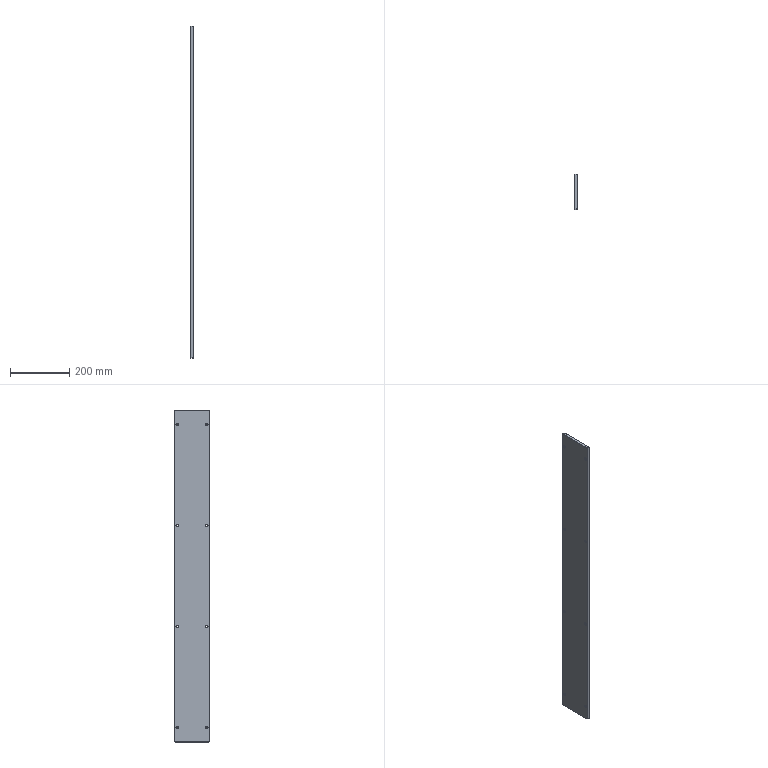Part | NX | 1 solid | 50 faces | box 10 x 118 x 1118 mm | volume 1313904 mm3 | cone 24 | plane 14 | cylinder 12 | commonest cylinder face diameters 6.5 x8 4 x4
STEP:
#1=CARTESIAN_POINT('',(-4.,57.,-559.));
#2=VERTEX_POINT('',#1);
#3=CARTESIAN_POINT('',(4.,57.,-559.));
#4=VERTEX_POINT('',#3);
#5=CARTESIAN_POINT('',(5.,57.,-559.));
#6=DIRECTION('',(-1.,0.,0.));
#7=VECTOR('',#6,1000.);
#8=LINE('',#5,#7);
#9=EDGE_CURVE('',#2,#4,#8,.F.);
#10=ORIENTED_EDGE('',*,*,#9,.T.);
#11=CARTESIAN_POINT('',(4.,-57.,-559.));
#12=VERTEX_POINT('',#11);
#13=CARTESIAN_POINT('',(4.,-59.,-559.));
#14=DIRECTION('',(0.,-1.,0.));
#15=VECTOR('',#14,1000.);
#16=LINE('',#13,#15);
#17=EDGE_CURVE('',#4,#12,#16,.T.);
#18=ORIENTED_EDGE('',*,*,#17,.T.);
#19=CARTESIAN_POINT('',(-4.,-57.,-559.));
#20=VERTEX_POINT('',#19);
#21=CARTESIAN_POINT('',(5.,-57.,-559.));
#22=DIRECTION('',(-1.,0.,0.));
#23=VECTOR('',#22,1000.);
#24=LINE('',#21,#23);
#25=EDGE_CURVE('',#12,#20,#24,.T.);
#26=ORIENTED_EDGE('',*,*,#25,.T.);
#27=CARTESIAN_POINT('',(-4.,57.,-559.));
#28=DIRECTION('',(0.,1.,0.));
#29=VECTOR('',#28,1000.);
#30=LINE('',#27,#29);
#31=EDGE_CURVE('',#20,#2,#30,.T.);
#32=ORIENTED_EDGE('',*,*,#31,.T.);
#33=EDGE_LOOP('',(#10,#18,#26,#32));
#34=FACE_BOUND('',#33,.T.);
#35=CARTESIAN_POINT('',(5.,-59.,-559.));
#36=DIRECTION('',(0.,0.,1.));
#37=DIRECTION('',(1.,0.,0.));
#38=AXIS2_PLACEMENT_3D('',#35,#36,#37);
#39=PLANE('',#38);
#40=ADVANCED_FACE('',(#34),#39,.F.);
#41=CARTESIAN_POINT('',(-4.,59.,557.));
#42=VERTEX_POINT('',#41);
#43=CARTESIAN_POINT('',(4.,59.,557.));
#44=VERTEX_POINT('',#43);
#45=CARTESIAN_POINT('',(5.,59.,557.));
#46=DIRECTION('',(-1.,0.,0.));
#47=VECTOR('',#46,1000.);
#48=LINE('',#45,#47);
#49=EDGE_CURVE('',#42,#44,#48,.F.);
#50=ORIENTED_EDGE('',*,*,#49,.T.);
#51=CARTESIAN_POINT('',(4.,59.,-557.));
#52=VERTEX_POINT('',#51);
#53=CARTESIAN_POINT('',(4.,59.,559.));
#54=DIRECTION('',(0.,0.,-1.));
#55=VECTOR('',#54,1000.);
#56=LINE('',#53,#55);
#57=EDGE_CURVE('',#44,#52,#56,.T.);
#58=ORIENTED_EDGE('',*,*,#57,.T.);
#59=CARTESIAN_POINT('',(-4.,59.,-557.));
#60=VERTEX_POINT('',#59);
#61=CARTESIAN_POINT('',(5.,59.,-557.));
#62=DIRECTION('',(-1.,0.,0.));
#63=VECTOR('',#62,1000.);
#64=LINE('',#61,#63);
#65=EDGE_CURVE('',#52,#60,#64,.T.);
#66=ORIENTED_EDGE('',*,*,#65,.T.);
#67=CARTESIAN_POINT('',(-4.,59.,557.));
#68=DIRECTION('',(0.,0.,1.));
#69=VECTOR('',#68,1000.);
#70=LINE('',#67,#69);
#71=EDGE_CURVE('',#60,#42,#70,.T.);
#72=ORIENTED_EDGE('',*,*,#71,.T.);
#73=EDGE_LOOP('',(#50,#58,#66,#72));
#74=FACE_BOUND('',#73,.T.);
#75=CARTESIAN_POINT('',(5.,59.,559.));
#76=DIRECTION('',(0.,-1.,0.));
#77=DIRECTION('',(0.,0.,-1.));
#78=AXIS2_PLACEMENT_3D('',#75,#76,#77);
#79=PLANE('',#78);
#80=ADVANCED_FACE('',(#74),#79,.F.);
#81=CARTESIAN_POINT('',(-4.,-57.,559.));
#82=VERTEX_POINT('',#81);
#83=CARTESIAN_POINT('',(4.,-57.,559.));
#84=VERTEX_POINT('',#83);
#85=CARTESIAN_POINT('',(5.,-57.,559.));
#86=DIRECTION('',(-1.,0.,0.));
#87=VECTOR('',#86,1000.);
#88=LINE('',#85,#87);
#89=EDGE_CURVE('',#82,#84,#88,.F.);
#90=ORIENTED_EDGE('',*,*,#89,.T.);
#91=CARTESIAN_POINT('',(4.,57.,559.));
#92=VERTEX_POINT('',#91);
#93=CARTESIAN_POINT('',(4.,-59.,559.));
#94=DIRECTION('',(0.,1.,0.));
#95=VECTOR('',#94,1000.);
#96=LINE('',#93,#95);
#97=EDGE_CURVE('',#84,#92,#96,.T.);
#98=ORIENTED_EDGE('',*,*,#97,.T.);
#99=CARTESIAN_POINT('',(-4.,57.,559.));
#100=VERTEX_POINT('',#99);
#101=CARTESIAN_POINT('',(5.,57.,559.));
#102=DIRECTION('',(-1.,0.,0.));
#103=VECTOR('',#102,1000.);
#104=LINE('',#101,#103);
#105=EDGE_CURVE('',#92,#100,#104,.T.);
#106=ORIENTED_EDGE('',*,*,#105,.T.);
#107=CARTESIAN_POINT('',(-4.,-57.,559.));
#108=DIRECTION('',(0.,-1.,0.));
#109=VECTOR('',#108,1000.);
#110=LINE('',#107,#109);
#111=EDGE_CURVE('',#100,#82,#110,.T.);
#112=ORIENTED_EDGE('',*,*,#111,.T.);
#113=EDGE_LOOP('',(#90,#98,#106,#112));
#114=FACE_BOUND('',#113,.T.);
#115=CARTESIAN_POINT('',(5.,-59.,559.));
#116=DIRECTION('',(0.,0.,-1.));
#117=DIRECTION('',(-1.,0.,0.));
#118=AXIS2_PLACEMENT_3D('',#115,#116,#117);
#119=PLANE('',#118);
#120=ADVANCED_FACE('',(#114),#119,.F.);
#121=CARTESIAN_POINT('',(-4.,-59.,-557.));
#122=VERTEX_POINT('',#121);
#123=CARTESIAN_POINT('',(4.,-59.,-557.));
#124=VERTEX_POINT('',#123);
#125=CARTESIAN_POINT('',(5.,-59.,-557.));
#126=DIRECTION('',(-1.,0.,0.));
#127=VECTOR('',#126,1000.);
#128=LINE('',#125,#127);
#129=EDGE_CURVE('',#122,#124,#128,.F.);
#130=ORIENTED_EDGE('',*,*,#129,.T.);
#131=CARTESIAN_POINT('',(4.,-59.,557.));
#132=VERTEX_POINT('',#131);
#133=CARTESIAN_POINT('',(4.,-59.,559.));
#134=DIRECTION('',(0.,0.,1.));
#135=VECTOR('',#134,1000.);
#136=LINE('',#133,#135);
#137=EDGE_CURVE('',#124,#132,#136,.T.);
#138=ORIENTED_EDGE('',*,*,#137,.T.);
#139=CARTESIAN_POINT('',(-4.,-59.,557.));
#140=VERTEX_POINT('',#139);
#141=CARTESIAN_POINT('',(5.,-59.,557.));
#142=DIRECTION('',(-1.,0.,0.));
#143=VECTOR('',#142,1000.);
#144=LINE('',#141,#143);
#145=EDGE_CURVE('',#132,#140,#144,.T.);
#146=ORIENTED_EDGE('',*,*,#145,.T.);
#147=CARTESIAN_POINT('',(-4.,-59.,-557.));
#148=DIRECTION('',(0.,0.,-1.));
#149=VECTOR('',#148,1000.);
#150=LINE('',#147,#149);
#151=EDGE_CURVE('',#140,#122,#150,.T.);
#152=ORIENTED_EDGE('',*,*,#151,.T.);
#153=EDGE_LOOP('',(#130,#138,#146,#152));
#154=FACE_BOUND('',#153,.T.);
#155=CARTESIAN_POINT('',(5.,-59.,559.));
#156=DIRECTION('',(0.,1.,0.));
#157=DIRECTION('',(0.,0.,1.));
#158=AXIS2_PLACEMENT_3D('',#155,#156,#157);
#159=PLANE('',#158);
#160=ADVANCED_FACE('',(#154),#159,.F.);
#161=CARTESIAN_POINT('',(5.,-58.,557.));
#162=VERTEX_POINT('',#161);
#163=CARTESIAN_POINT('',(5.,-58.,-557.));
#164=VERTEX_POINT('',#163);
#165=CARTESIAN_POINT('',(5.,-58.,0.));
#166=DIRECTION('',(0.,0.,-1.));
#167=VECTOR('',#166,1000.);
#168=LINE('',#165,#167);
#169=EDGE_CURVE('',#162,#164,#168,.T.);
#170=ORIENTED_EDGE('',*,*,#169,.T.);
#171=CARTESIAN_POINT('',(5.,-57.,-558.));
#172=VERTEX_POINT('',#171);
#173=CARTESIAN_POINT('',(5.,-57.,-557.));
#174=DIRECTION('',(-1.,0.,0.));
#175=DIRECTION('',(0.,0.,1.));
#176=AXIS2_PLACEMENT_3D('',#173,#174,#175);
#177=CIRCLE('',#176,1.);
#178=EDGE_CURVE('',#164,#172,#177,.F.);
#179=ORIENTED_EDGE('',*,*,#178,.T.);
#180=CARTESIAN_POINT('',(5.,57.,-558.));
#181=VERTEX_POINT('',#180);
#182=CARTESIAN_POINT('',(5.,0.,-558.));
#183=DIRECTION('',(0.,1.,0.));
#184=VECTOR('',#183,1000.);
#185=LINE('',#182,#184);
#186=EDGE_CURVE('',#172,#181,#185,.T.);
#187=ORIENTED_EDGE('',*,*,#186,.T.);
#188=CARTESIAN_POINT('',(5.,58.,-557.));
#189=VERTEX_POINT('',#188);
#190=CARTESIAN_POINT('',(5.,57.,-557.));
#191=DIRECTION('',(-1.,0.,0.));
#192=DIRECTION('',(0.,0.,1.));
#193=AXIS2_PLACEMENT_3D('',#190,#191,#192);
#194=CIRCLE('',#193,1.);
#195=EDGE_CURVE('',#181,#189,#194,.F.);
#196=ORIENTED_EDGE('',*,*,#195,.T.);
#197=CARTESIAN_POINT('',(5.,58.,557.));
#198=VERTEX_POINT('',#197);
#199=CARTESIAN_POINT('',(5.,58.,0.));
#200=DIRECTION('',(0.,0.,1.));
#201=VECTOR('',#200,1000.);
#202=LINE('',#199,#201);
#203=EDGE_CURVE('',#189,#198,#202,.T.);
#204=ORIENTED_EDGE('',*,*,#203,.T.);
#205=CARTESIAN_POINT('',(5.,57.,558.));
#206=VERTEX_POINT('',#205);
#207=CARTESIAN_POINT('',(5.,57.,557.));
#208=DIRECTION('',(-1.,0.,0.));
#209=DIRECTION('',(0.,0.,1.));
#210=AXIS2_PLACEMENT_3D('',#207,#208,#209);
#211=CIRCLE('',#210,1.);
#212=EDGE_CURVE('',#198,#206,#211,.F.);
#213=ORIENTED_EDGE('',*,*,#212,.T.);
#214=CARTESIAN_POINT('',(5.,-57.,558.));
#215=VERTEX_POINT('',#214);
#216=CARTESIAN_POINT('',(5.,0.,558.));
#217=DIRECTION('',(0.,-1.,0.));
#218=VECTOR('',#217,1000.);
#219=LINE('',#216,#218);
#220=EDGE_CURVE('',#206,#215,#219,.T.);
#221=ORIENTED_EDGE('',*,*,#220,.T.);
#222=CARTESIAN_POINT('',(5.,-57.,557.));
#223=DIRECTION('',(-1.,0.,0.));
#224=DIRECTION('',(0.,0.,1.));
#225=AXIS2_PLACEMENT_3D('',#222,#223,#224);
#226=CIRCLE('',#225,1.);
#227=EDGE_CURVE('',#215,#162,#226,.F.);
#228=ORIENTED_EDGE('',*,*,#227,.T.);
#229=EDGE_LOOP('',(#170,#179,#187,#196,#204,#213,#221,#228));
#230=FACE_BOUND('',#229,.T.);
#231=CARTESIAN_POINT('',(5.,-50.,-505.75));
#232=VERTEX_POINT('',#231);
#233=CARTESIAN_POINT('',(5.,-50.,-510.));
#234=DIRECTION('',(-1.,0.,0.));
#235=DIRECTION('',(0.,0.,1.));
#236=AXIS2_PLACEMENT_3D('',#233,#234,#235);
#237=CIRCLE('',#236,4.25);
#238=EDGE_CURVE('',#232,#232,#237,.T.);
#239=ORIENTED_EDGE('',*,*,#238,.T.);
#240=EDGE_LOOP('',(#239));
#241=FACE_BOUND('',#240,.T.);
#242=CARTESIAN_POINT('',(5.,-50.,-165.75));
#243=VERTEX_POINT('',#242);
#244=CARTESIAN_POINT('',(5.,-50.,-170.));
#245=DIRECTION('',(-1.,0.,0.));
#246=DIRECTION('',(0.,0.,1.));
#247=AXIS2_PLACEMENT_3D('',#244,#245,#246);
#248=CIRCLE('',#247,4.25);
#249=EDGE_CURVE('',#243,#243,#248,.T.);
#250=ORIENTED_EDGE('',*,*,#249,.T.);
#251=EDGE_LOOP('',(#250));
#252=FACE_BOUND('',#251,.T.);
#253=CARTESIAN_POINT('',(5.,-50.,174.25));
#254=VERTEX_POINT('',#253);
#255=CARTESIAN_POINT('',(5.,-50.,170.));
#256=DIRECTION('',(-1.,0.,0.));
#257=DIRECTION('',(0.,0.,1.));
#258=AXIS2_PLACEMENT_3D('',#255,#256,#257);
#259=CIRCLE('',#258,4.25);
#260=EDGE_CURVE('',#254,#254,#259,.T.);
#261=ORIENTED_EDGE('',*,*,#260,.T.);
#262=EDGE_LOOP('',(#261));
#263=FACE_BOUND('',#262,.T.);
#264=CARTESIAN_POINT('',(5.,-50.,514.25));
#265=VERTEX_POINT('',#264);
#266=CARTESIAN_POINT('',(5.,-50.,510.));
#267=DIRECTION('',(-1.,0.,0.));
#268=DIRECTION('',(0.,0.,1.));
#269=AXIS2_PLACEMENT_3D('',#266,#267,#268);
#270=CIRCLE('',#269,4.25);
#271=EDGE_CURVE('',#265,#265,#270,.T.);
#272=ORIENTED_EDGE('',*,*,#271,.T.);
#273=EDGE_LOOP('',(#272));
#274=FACE_BOUND('',#273,.T.);
#275=CARTESIAN_POINT('',(5.,50.,174.25));
#276=VERTEX_POINT('',#275);
#277=CARTESIAN_POINT('',(5.,50.,170.));
#278=DIRECTION('',(-1.,0.,0.));
#279=DIRECTION('',(0.,0.,1.));
#280=AXIS2_PLACEMENT_3D('',#277,#278,#279);
#281=CIRCLE('',#280,4.25);
#282=EDGE_CURVE('',#276,#276,#281,.T.);
#283=ORIENTED_EDGE('',*,*,#282,.T.);
#284=EDGE_LOOP('',(#283));
#285=FACE_BOUND('',#284,.T.);
#286=CARTESIAN_POINT('',(5.,50.,514.25));
#287=VERTEX_POINT('',#286);
#288=CARTESIAN_POINT('',(5.,50.,510.));
#289=DIRECTION('',(-1.,0.,0.));
#290=DIRECTION('',(0.,0.,1.));
#291=AXIS2_PLACEMENT_3D('',#288,#289,#290);
#292=CIRCLE('',#291,4.25);
#293=EDGE_CURVE('',#287,#287,#292,.T.);
#294=ORIENTED_EDGE('',*,*,#293,.T.);
#295=EDGE_LOOP('',(#294));
#296=FACE_BOUND('',#295,.T.);
#297=CARTESIAN_POINT('',(5.,50.,-505.75));
#298=VERTEX_POINT('',#297);
#299=CARTESIAN_POINT('',(5.,50.,-510.));
#300=DIRECTION('',(-1.,0.,0.));
#301=DIRECTION('',(0.,0.,1.));
#302=AXIS2_PLACEMENT_3D('',#299,#300,#301);
#303=CIRCLE('',#302,4.25);
#304=EDGE_CURVE('',#298,#298,#303,.T.);
#305=ORIENTED_EDGE('',*,*,#304,.T.);
#306=EDGE_LOOP('',(#305));
#307=FACE_BOUND('',#306,.T.);
#308=CARTESIAN_POINT('',(5.,50.,-165.75));
#309=VERTEX_POINT('',#308);
#310=CARTESIAN_POINT('',(5.,50.,-170.));
#311=DIRECTION('',(-1.,0.,0.));
#312=DIRECTION('',(0.,0.,1.));
#313=AXIS2_PLACEMENT_3D('',#310,#311,#312);
#314=CIRCLE('',#313,4.25);
#315=EDGE_CURVE('',#309,#309,#314,.T.);
#316=ORIENTED_EDGE('',*,*,#315,.T.);
#317=EDGE_LOOP('',(#316));
#318=FACE_BOUND('',#317,.T.);
#319=CARTESIAN_POINT('',(5.,0.,0.));
#320=DIRECTION('',(-1.,0.,0.));
#321=DIRECTION('',(0.,0.,1.));
#322=AXIS2_PLACEMENT_3D('',#319,#320,#321);
#323=PLANE('',#322);
#324=ADVANCED_FACE('',(#230,#241,#252,#263,#274,#285,#296,#307,#318),#323,.F.);
#325=CARTESIAN_POINT('',(-5.,-57.,558.));
#326=VERTEX_POINT('',#325);
#327=CARTESIAN_POINT('',(-5.,57.,558.));
#328=VERTEX_POINT('',#327);
#329=CARTESIAN_POINT('',(-5.,57.,558.));
#330=DIRECTION('',(0.,1.,0.));
#331=VECTOR('',#330,1000.);
#332=LINE('',#329,#331);
#333=EDGE_CURVE('',#326,#328,#332,.T.);
#334=ORIENTED_EDGE('',*,*,#333,.T.);
#335=CARTESIAN_POINT('',(-5.,58.,557.));
#336=VERTEX_POINT('',#335);
#337=CARTESIAN_POINT('',(-5.,57.,557.));
#338=DIRECTION('',(-1.,0.,0.));
#339=DIRECTION('',(0.,0.,1.));
#340=AXIS2_PLACEMENT_3D('',#337,#338,#339);
#341=CIRCLE('',#340,1.);
#342=EDGE_CURVE('',#328,#336,#341,.T.);
#343=ORIENTED_EDGE('',*,*,#342,.T.);
#344=CARTESIAN_POINT('',(-5.,58.,-557.));
#345=VERTEX_POINT('',#344);
#346=CARTESIAN_POINT('',(-5.,58.,-557.));
#347=DIRECTION('',(0.,0.,-1.));
#348=VECTOR('',#347,1000.);
#349=LINE('',#346,#348);
#350=EDGE_CURVE('',#336,#345,#349,.T.);
#351=ORIENTED_EDGE('',*,*,#350,.T.);
#352=CARTESIAN_POINT('',(-5.,57.,-558.));
#353=VERTEX_POINT('',#352);
#354=CARTESIAN_POINT('',(-5.,57.,-557.));
#355=DIRECTION('',(-1.,0.,0.));
#356=DIRECTION('',(0.,0.,1.));
#357=AXIS2_PLACEMENT_3D('',#354,#355,#356);
#358=CIRCLE('',#357,1.);
#359=EDGE_CURVE('',#345,#353,#358,.T.);
#360=ORIENTED_EDGE('',*,*,#359,.T.);
#361=CARTESIAN_POINT('',(-5.,-57.,-558.));
#362=VERTEX_POINT('',#361);
#363=CARTESIAN_POINT('',(-5.,-57.,-558.));
#364=DIRECTION('',(0.,-1.,0.));
#365=VECTOR('',#364,1000.);
#366=LINE('',#363,#365);
#367=EDGE_CURVE('',#353,#362,#366,.T.);
#368=ORIENTED_EDGE('',*,*,#367,.T.);
#369=CARTESIAN_POINT('',(-5.,-58.,-557.));
#370=VERTEX_POINT('',#369);
#371=CARTESIAN_POINT('',(-5.,-57.,-557.));
#372=DIRECTION('',(-1.,0.,0.));
#373=DIRECTION('',(0.,0.,1.));
#374=AXIS2_PLACEMENT_3D('',#371,#372,#373);
#375=CIRCLE('',#374,1.);
#376=EDGE_CURVE('',#362,#370,#375,.T.);
#377=ORIENTED_EDGE('',*,*,#376,.T.);
#378=CARTESIAN_POINT('',(-5.,-58.,557.));
#379=VERTEX_POINT('',#378);
#380=CARTESIAN_POINT('',(-5.,-58.,557.));
#381=DIRECTION('',(0.,0.,1.));
#382=VECTOR('',#381,1000.);
#383=LINE('',#380,#382);
#384=EDGE_CURVE('',#370,#379,#383,.T.);
#385=ORIENTED_EDGE('',*,*,#384,.T.);
#386=CARTESIAN_POINT('',(-5.,-57.,557.));
#387=DIRECTION('',(-1.,0.,0.));
#388=DIRECTION('',(0.,0.,1.));
#389=AXIS2_PLACEMENT_3D('',#386,#387,#388);
#390=CIRCLE('',#389,1.);
#391=EDGE_CURVE('',#379,#326,#390,.T.);
#392=ORIENTED_EDGE('',*,*,#391,.T.);
#393=EDGE_LOOP('',(#334,#343,#351,#360,#368,#377,#385,#392));
#394=FACE_BOUND('',#393,.T.);
#395=CARTESIAN_POINT('',(-5.,-50.,-505.75));
#396=VERTEX_POINT('',#395);
#397=CARTESIAN_POINT('',(-5.,-50.,-510.));
#398=DIRECTION('',(-1.,0.,0.));
#399=DIRECTION('',(0.,0.,1.));
#400=AXIS2_PLACEMENT_3D('',#397,#398,#399);
#401=CIRCLE('',#400,4.25);
#402=EDGE_CURVE('',#396,#396,#401,.F.);
#403=ORIENTED_EDGE('',*,*,#402,.T.);
#404=EDGE_LOOP('',(#403));
#405=FACE_BOUND('',#404,.T.);
#406=CARTESIAN_POINT('',(-5.,-50.,-165.75));
#407=VERTEX_POINT('',#406);
#408=CARTESIAN_POINT('',(-5.,-50.,-170.));
#409=DIRECTION('',(-1.,0.,0.));
#410=DIRECTION('',(0.,0.,1.));
#411=AXIS2_PLACEMENT_3D('',#408,#409,#410);
#412=CIRCLE('',#411,4.25);
#413=EDGE_CURVE('',#407,#407,#412,.F.);
#414=ORIENTED_EDGE('',*,*,#413,.T.);
#415=EDGE_LOOP('',(#414));
#416=FACE_BOUND('',#415,.T.);
#417=CARTESIAN_POINT('',(-5.,-50.,174.25));
#418=VERTEX_POINT('',#417);
#419=CARTESIAN_POINT('',(-5.,-50.,170.));
#420=DIRECTION('',(-1.,0.,0.));
#421=DIRECTION('',(0.,0.,1.));
#422=AXIS2_PLACEMENT_3D('',#419,#420,#421);
#423=CIRCLE('',#422,4.25);
#424=EDGE_CURVE('',#418,#418,#423,.F.);
#425=ORIENTED_EDGE('',*,*,#424,.T.);
#426=EDGE_LOOP('',(#425));
#427=FACE_BOUND('',#426,.T.);
#428=CARTESIAN_POINT('',(-5.,-50.,514.25));
#429=VERTEX_POINT('',#428);
#430=CARTESIAN_POINT('',(-5.,-50.,510.));
#431=DIRECTION('',(-1.,0.,0.));
#432=DIRECTION('',(0.,0.,1.));
#433=AXIS2_PLACEMENT_3D('',#430,#431,#432);
#434=CIRCLE('',#433,4.25);
#435=EDGE_CURVE('',#429,#429,#434,.F.);
#436=ORIENTED_EDGE('',*,*,#435,.T.);
#437=EDGE_LOOP('',(#436));
#438=FACE_BOUND('',#437,.T.);
#439=CARTESIAN_POINT('',(-5.,50.,174.25));
#440=VERTEX_POINT('',#439);
#441=CARTESIAN_POINT('',(-5.,50.,170.));
#442=DIRECTION('',(-1.,0.,0.));
#443=DIRECTION('',(0.,0.,1.));
#444=AXIS2_PLACEMENT_3D('',#441,#442,#443);
#445=CIRCLE('',#444,4.25);
#446=EDGE_CURVE('',#440,#440,#445,.F.);
#447=ORIENTED_EDGE('',*,*,#446,.T.);
#448=EDGE_LOOP('',(#447));
#449=FACE_BOUND('',#448,.T.);
#450=CARTESIAN_POINT('',(-5.,50.,514.25));
#451=VERTEX_POINT('',#450);
#452=CARTESIAN_POINT('',(-5.,50.,510.));
#453=DIRECTION('',(-1.,0.,0.));
#454=DIRECTION('',(0.,0.,1.));
#455=AXIS2_PLACEMENT_3D('',#452,#453,#454);
#456=CIRCLE('',#455,4.25);
#457=EDGE_CURVE('',#451,#451,#456,.F.);
#458=ORIENTED_EDGE('',*,*,#457,.T.);
#459=EDGE_LOOP('',(#458));
#460=FACE_BOUND('',#459,.T.);
#461=CARTESIAN_POINT('',(-5.,50.,-505.75));
#462=VERTEX_POINT('',#461);
#463=CARTESIAN_POINT('',(-5.,50.,-510.));
#464=DIRECTION('',(-1.,0.,0.));
#465=DIRECTION('',(0.,0.,1.));
#466=AXIS2_PLACEMENT_3D('',#463,#464,#465);
#467=CIRCLE('',#466,4.25);
#468=EDGE_CURVE('',#462,#462,#467,.F.);
#469=ORIENTED_EDGE('',*,*,#468,.T.);
#470=EDGE_LOOP('',(#469));
#471=FACE_BOUND('',#470,.T.);
#472=CARTESIAN_POINT('',(-5.,50.,-165.75));
#473=VERTEX_POINT('',#472);
#474=CARTESIAN_POINT('',(-5.,50.,-170.));
#475=DIRECTION('',(-1.,0.,0.));
#476=DIRECTION('',(0.,0.,1.));
#477=AXIS2_PLACEMENT_3D('',#474,#475,#476);
#478=CIRCLE('',#477,4.25);
#479=EDGE_CURVE('',#473,#473,#478,.F.);
#480=ORIENTED_EDGE('',*,*,#479,.T.);
#481=EDGE_LOOP('',(#480));
#482=FACE_BOUND('',#481,.T.);
#483=CARTESIAN_POINT('',(-5.,0.,0.));
#484=DIRECTION('',(-1.,0.,0.));
#485=DIRECTION('',(0.,0.,1.));
#486=AXIS2_PLACEMENT_3D('',#483,#484,#485);
#487=PLANE('',#486);
#488=ADVANCED_FACE('',(#394,#405,#416,#427,#438,#449,#460,#471,#482),#487,.T.);
#489=CARTESIAN_POINT('',(4.,-50.,-506.75));
#490=VERTEX_POINT('',#489);
#491=CARTESIAN_POINT('',(4.,-50.,-510.));
#492=DIRECTION('',(-1.,0.,0.));
#493=DIRECTION('',(0.,0.,1.));
#494=AXIS2_PLACEMENT_3D('',#491,#492,#493);
#495=CIRCLE('',#494,3.25);
#496=EDGE_CURVE('',#490,#490,#495,.F.);
#497=ORIENTED_EDGE('',*,*,#496,.T.);
#498=EDGE_LOOP('',(#497));
#499=FACE_BOUND('',#498,.T.);
#500=CARTESIAN_POINT('',(-4.,-50.,-506.75));
#501=VERTEX_POINT('',#500);
#502=CARTESIAN_POINT('',(-4.,-50.,-510.));
#503=DIRECTION('',(-1.,0.,0.));
#504=DIRECTION('',(0.,0.,1.));
#505=AXIS2_PLACEMENT_3D('',#502,#503,#504);
#506=CIRCLE('',#505,3.25);
#507=EDGE_CURVE('',#501,#501,#506,.T.);
#508=ORIENTED_EDGE('',*,*,#507,.T.);
#509=EDGE_LOOP('',(#508));
#510=FACE_BOUND('',#509,.T.);
#511=CARTESIAN_POINT('',(5.,-50.,-510.));
#512=DIRECTION('',(1.,0.,0.));
#513=DIRECTION('',(0.,0.,-1.));
#514=AXIS2_PLACEMENT_3D('',#511,#512,#513);
#515=CYLINDRICAL_SURFACE('',#514,3.25);
#516=ADVANCED_FACE('',(#499,#510),#515,.F.);
#517=CARTESIAN_POINT('',(4.,-50.,-166.75));
#518=VERTEX_POINT('',#517);
#519=CARTESIAN_POINT('',(4.,-50.,-170.));
#520=DIRECTION('',(-1.,0.,0.));
#521=DIRECTION('',(0.,0.,1.));
#522=AXIS2_PLACEMENT_3D('',#519,#520,#521);
#523=CIRCLE('',#522,3.25);
#524=EDGE_CURVE('',#518,#518,#523,.F.);
#525=ORIENTED_EDGE('',*,*,#524,.T.);
#526=EDGE_LOOP('',(#525));
#527=FACE_BOUND('',#526,.T.);
#528=CARTESIAN_POINT('',(-4.,-50.,-166.75));
#529=VERTEX_POINT('',#528);
#530=CARTESIAN_POINT('',(-4.,-50.,-170.));
#531=DIRECTION('',(-1.,0.,0.));
#532=DIRECTION('',(0.,0.,1.));
#533=AXIS2_PLACEMENT_3D('',#530,#531,#532);
#534=CIRCLE('',#533,3.25);
#535=EDGE_CURVE('',#529,#529,#534,.T.);
#536=ORIENTED_EDGE('',*,*,#535,.T.);
#537=EDGE_LOOP('',(#536));
#538=FACE_BOUND('',#537,.T.);
#539=CARTESIAN_POINT('',(5.,-50.,-170.));
#540=DIRECTION('',(1.,0.,0.));
#541=DIRECTION('',(0.,0.,-1.));
#542=AXIS2_PLACEMENT_3D('',#539,#540,#541);
#543=CYLINDRICAL_SURFACE('',#542,3.25);
#544=ADVANCED_FACE('',(#527,#538),#543,.F.);
#545=CARTESIAN_POINT('',(4.,-50.,173.25));
#546=VERTEX_POINT('',#545);
#547=CARTESIAN_POINT('',(4.,-50.,170.));
#548=DIRECTION('',(-1.,0.,0.));
#549=DIRECTION('',(0.,0.,1.));
#550=AXIS2_PLACEMENT_3D('',#547,#548,#549);
#551=CIRCLE('',#550,3.25);
#552=EDGE_CURVE('',#546,#546,#551,.F.);
#553=ORIENTED_EDGE('',*,*,#552,.T.);
#554=EDGE_LOOP('',(#553));
#555=FACE_BOUND('',#554,.T.);
#556=CARTESIAN_POINT('',(-4.,-50.,173.25));
#557=VERTEX_POINT('',#556);
#558=CARTESIAN_POINT('',(-4.,-50.,170.));
#559=DIRECTION('',(-1.,0.,0.));
#560=DIRECTION('',(0.,0.,1.));
#561=AXIS2_PLACEMENT_3D('',#558,#559,#560);
#562=CIRCLE('',#561,3.25);
#563=EDGE_CURVE('',#557,#557,#562,.T.);
#564=ORIENTED_EDGE('',*,*,#563,.T.);
#565=EDGE_LOOP('',(#564));
#566=FACE_BOUND('',#565,.T.);
#567=CARTESIAN_POINT('',(5.,-50.,170.));
#568=DIRECTION('',(1.,0.,0.));
#569=DIRECTION('',(0.,0.,-1.));
#570=AXIS2_PLACEMENT_3D('',#567,#568,#569);
#571=CYLINDRICAL_SURFACE('',#570,3.25);
#572=ADVANCED_FACE('',(#555,#566),#571,.F.);
#573=CARTESIAN_POINT('',(4.,-50.,513.25));
#574=VERTEX_POINT('',#573);
#575=CARTESIAN_POINT('',(4.,-50.,510.));
#576=DIRECTION('',(-1.,0.,0.));
#577=DIRECTION('',(0.,0.,1.));
#578=AXIS2_PLACEMENT_3D('',#575,#576,#577);
#579=CIRCLE('',#578,3.25);
#580=EDGE_CURVE('',#574,#574,#579,.F.);
#581=ORIENTED_EDGE('',*,*,#580,.T.);
#582=EDGE_LOOP('',(#581));
#583=FACE_BOUND('',#582,.T.);
#584=CARTESIAN_POINT('',(-4.,-50.,513.25));
#585=VERTEX_POINT('',#584);
#586=CARTESIAN_POINT('',(-4.,-50.,510.));
#587=DIRECTION('',(-1.,0.,0.));
#588=DIRECTION('',(0.,0.,1.));
#589=AXIS2_PLACEMENT_3D('',#586,#587,#588);
#590=CIRCLE('',#589,3.25);
#591=EDGE_CURVE('',#585,#585,#590,.T.);
#592=ORIENTED_EDGE('',*,*,#591,.T.);
#593=EDGE_LOOP('',(#592));
#594=FACE_BOUND('',#593,.T.);
#595=CARTESIAN_POINT('',(5.,-50.,510.));
#596=DIRECTION('',(1.,0.,0.));
#597=DIRECTION('',(0.,0.,-1.));
#598=AXIS2_PLACEMENT_3D('',#595,#596,#597);
#599=CYLINDRICAL_SURFACE('',#598,3.25);
#600=ADVANCED_FACE('',(#583,#594),#599,.F.);
#601=CARTESIAN_POINT('',(4.,50.,173.25));
#602=VERTEX_POINT('',#601);
#603=CARTESIAN_POINT('',(4.,50.,170.));
#604=DIRECTION('',(-1.,0.,0.));
#605=DIRECTION('',(0.,0.,1.));
#606=AXIS2_PLACEMENT_3D('',#603,#604,#605);
#607=CIRCLE('',#606,3.25);
#608=EDGE_CURVE('',#602,#602,#607,.F.);
#609=ORIENTED_EDGE('',*,*,#608,.T.);
#610=EDGE_LOOP('',(#609));
#611=FACE_BOUND('',#610,.T.);
#612=CARTESIAN_POINT('',(-4.,50.,173.25));
#613=VERTEX_POINT('',#612);
#614=CARTESIAN_POINT('',(-4.,50.,170.));
#615=DIRECTION('',(-1.,0.,0.));
#616=DIRECTION('',(0.,0.,1.));
#617=AXIS2_PLACEMENT_3D('',#614,#615,#616);
#618=CIRCLE('',#617,3.25);
#619=EDGE_CURVE('',#613,#613,#618,.T.);
#620=ORIENTED_EDGE('',*,*,#619,.T.);
#621=EDGE_LOOP('',(#620));
#622=FACE_BOUND('',#621,.T.);
#623=CARTESIAN_POINT('',(5.,50.,170.));
#624=DIRECTION('',(1.,0.,0.));
#625=DIRECTION('',(0.,0.,-1.));
#626=AXIS2_PLACEMENT_3D('',#623,#624,#625);
#627=CYLINDRICAL_SURFACE('',#626,3.25);
#628=ADVANCED_FACE('',(#611,#622),#627,.F.);
#629=CARTESIAN_POINT('',(4.,50.,513.25));
#630=VERTEX_POINT('',#629);
#631=CARTESIAN_POINT('',(4.,50.,510.));
#632=DIRECTION('',(-1.,0.,0.));
#633=DIRECTION('',(0.,0.,1.));
#634=AXIS2_PLACEMENT_3D('',#631,#632,#633);
#635=CIRCLE('',#634,3.25);
#636=EDGE_CURVE('',#630,#630,#635,.F.);
#637=ORIENTED_EDGE('',*,*,#636,.T.);
#638=EDGE_LOOP('',(#637));
#639=FACE_BOUND('',#638,.T.);
#640=CARTESIAN_POINT('',(-4.,50.,513.25));
#641=VERTEX_POINT('',#640);
#642=CARTESIAN_POINT('',(-4.,50.,510.));
#643=DIRECTION('',(-1.,0.,0.));
#644=DIRECTION('',(0.,0.,1.));
#645=AXIS2_PLACEMENT_3D('',#642,#643,#644);
#646=CIRCLE('',#645,3.25);
#647=EDGE_CURVE('',#641,#641,#646,.T.);
#648=ORIENTED_EDGE('',*,*,#647,.T.);
#649=EDGE_LOOP('',(#648));
#650=FACE_BOUND('',#649,.T.);
#651=CARTESIAN_POINT('',(5.,50.,510.));
#652=DIRECTION('',(1.,0.,0.));
#653=DIRECTION('',(0.,0.,-1.));
#654=AXIS2_PLACEMENT_3D('',#651,#652,#653);
#655=CYLINDRICAL_SURFACE('',#654,3.25);
#656=ADVANCED_FACE('',(#639,#650),#655,.F.);
#657=CARTESIAN_POINT('',(4.,50.,-506.75));
#658=VERTEX_POINT('',#657);
#659=CARTESIAN_POINT('',(4.,50.,-510.));
#660=DIRECTION('',(-1.,0.,0.));
#661=DIRECTION('',(0.,0.,1.));
#662=AXIS2_PLACEMENT_3D('',#659,#660,#661);
#663=CIRCLE('',#662,3.25);
#664=EDGE_CURVE('',#658,#658,#663,.F.);
#665=ORIENTED_EDGE('',*,*,#664,.T.);
#666=EDGE_LOOP('',(#665));
#667=FACE_BOUND('',#666,.T.);
#668=CARTESIAN_POINT('',(-4.,50.,-506.75));
#669=VERTEX_POINT('',#668);
#670=CARTESIAN_POINT('',(-4.,50.,-510.));
#671=DIRECTION('',(-1.,0.,0.));
#672=DIRECTION('',(0.,0.,1.));
#673=AXIS2_PLACEMENT_3D('',#670,#671,#672);
#674=CIRCLE('',#673,3.25);
#675=EDGE_CURVE('',#669,#669,#674,.T.);
#676=ORIENTED_EDGE('',*,*,#675,.T.);
#677=EDGE_LOOP('',(#676));
#678=FACE_BOUND('',#677,.T.);
#679=CARTESIAN_POINT('',(5.,50.,-510.));
#680=DIRECTION('',(1.,0.,0.));
#681=DIRECTION('',(0.,0.,-1.));
#682=AXIS2_PLACEMENT_3D('',#679,#680,#681);
#683=CYLINDRICAL_SURFACE('',#682,3.25);
#684=ADVANCED_FACE('',(#667,#678),#683,.F.);
#685=CARTESIAN_POINT('',(4.,50.,-166.75));
#686=VERTEX_POINT('',#685);
#687=CARTESIAN_POINT('',(4.,50.,-170.));
#688=DIRECTION('',(-1.,0.,0.));
#689=DIRECTION('',(0.,0.,1.));
#690=AXIS2_PLACEMENT_3D('',#687,#688,#689);
#691=CIRCLE('',#690,3.25);
#692=EDGE_CURVE('',#686,#686,#691,.F.);
#693=ORIENTED_EDGE('',*,*,#692,.T.);
#694=EDGE_LOOP('',(#693));
#695=FACE_BOUND('',#694,.T.);
#696=CARTESIAN_POINT('',(-4.,50.,-166.75));
#697=VERTEX_POINT('',#696);
#698=CARTESIAN_POINT('',(-4.,50.,-170.));
#699=DIRECTION('',(-1.,0.,0.));
#700=DIRECTION('',(0.,0.,1.));
#701=AXIS2_PLACEMENT_3D('',#698,#699,#700);
#702=CIRCLE('',#701,3.25);
#703=EDGE_CURVE('',#697,#697,#702,.T.);
#704=ORIENTED_EDGE('',*,*,#703,.T.);
#705=EDGE_LOOP('',(#704));
#706=FACE_BOUND('',#705,.T.);
#707=CARTESIAN_POINT('',(5.,50.,-170.));
#708=DIRECTION('',(1.,0.,0.));
#709=DIRECTION('',(0.,0.,-1.));
#710=AXIS2_PLACEMENT_3D('',#707,#708,#709);
#711=CYLINDRICAL_SURFACE('',#710,3.25);
#712=ADVANCED_FACE('',(#695,#706),#711,.F.);
#713=ORIENTED_EDGE('',*,*,#65,.F.);
#714=CARTESIAN_POINT('',(4.,57.,-557.));
#715=DIRECTION('',(-1.,0.,0.));
#716=DIRECTION('',(0.,0.,1.));
#717=AXIS2_PLACEMENT_3D('',#714,#715,#716);
#718=CIRCLE('',#717,2.);
#719=EDGE_CURVE('',#52,#4,#718,.T.);
#720=ORIENTED_EDGE('',*,*,#719,.T.);
#721=ORIENTED_EDGE('',*,*,#9,.F.);
#722=CARTESIAN_POINT('',(-4.,57.,-557.));
#723=DIRECTION('',(-1.,0.,0.));
#724=DIRECTION('',(0.,0.,1.));
#725=AXIS2_PLACEMENT_3D('',#722,#723,#724);
#726=CIRCLE('',#725,2.);
#727=EDGE_CURVE('',#2,#60,#726,.F.);
#728=ORIENTED_EDGE('',*,*,#727,.T.);
#729=EDGE_LOOP('',(#713,#720,#721,#728));
#730=FACE_BOUND('',#729,.T.);
#731=CARTESIAN_POINT('',(5.,57.,-557.));
#732=DIRECTION('',(-1.,0.,0.));
#733=DIRECTION('',(0.,0.,1.));
#734=AXIS2_PLACEMENT_3D('',#731,#732,#733);
#735=CYLINDRICAL_SURFACE('',#734,2.);
#736=ADVANCED_FACE('',(#730),#735,.T.);
#737=ORIENTED_EDGE('',*,*,#25,.F.);
#738=CARTESIAN_POINT('',(4.,-57.,-557.));
#739=DIRECTION('',(-1.,0.,0.));
#740=DIRECTION('',(0.,0.,1.));
#741=AXIS2_PLACEMENT_3D('',#738,#739,#740);
#742=CIRCLE('',#741,2.);
#743=EDGE_CURVE('',#12,#124,#742,.T.);
#744=ORIENTED_EDGE('',*,*,#743,.T.);
#745=ORIENTED_EDGE('',*,*,#129,.F.);
#746=CARTESIAN_POINT('',(-4.,-57.,-557.));
#747=DIRECTION('',(-1.,0.,0.));
#748=DIRECTION('',(0.,0.,1.));
#749=AXIS2_PLACEMENT_3D('',#746,#747,#748);
#750=CIRCLE('',#749,2.);
#751=EDGE_CURVE('',#122,#20,#750,.F.);
#752=ORIENTED_EDGE('',*,*,#751,.T.);
#753=EDGE_LOOP('',(#737,#744,#745,#752));
#754=FACE_BOUND('',#753,.T.);
#755=CARTESIAN_POINT('',(5.,-57.,-557.));
#756=DIRECTION('',(-1.,0.,0.));
#757=DIRECTION('',(0.,0.,1.));
#758=AXIS2_PLACEMENT_3D('',#755,#756,#757);
#759=CYLINDRICAL_SURFACE('',#758,2.);
#760=ADVANCED_FACE('',(#754),#759,.T.);
#761=ORIENTED_EDGE('',*,*,#145,.F.);
#762=CARTESIAN_POINT('',(4.,-57.,557.));
#763=DIRECTION('',(-1.,0.,0.));
#764=DIRECTION('',(0.,0.,1.));
#765=AXIS2_PLACEMENT_3D('',#762,#763,#764);
#766=CIRCLE('',#765,2.);
#767=EDGE_CURVE('',#132,#84,#766,.T.);
#768=ORIENTED_EDGE('',*,*,#767,.T.);
#769=ORIENTED_EDGE('',*,*,#89,.F.);
#770=CARTESIAN_POINT('',(-4.,-57.,557.));
#771=DIRECTION('',(-1.,0.,0.));
#772=DIRECTION('',(0.,0.,1.));
#773=AXIS2_PLACEMENT_3D('',#770,#771,#772);
#774=CIRCLE('',#773,2.);
#775=EDGE_CURVE('',#82,#140,#774,.F.);
#776=ORIENTED_EDGE('',*,*,#775,.T.);
#777=EDGE_LOOP('',(#761,#768,#769,#776));
#778=FACE_BOUND('',#777,.T.);
#779=CARTESIAN_POINT('',(5.,-57.,557.));
#780=DIRECTION('',(-1.,0.,0.));
#781=DIRECTION('',(0.,0.,1.));
#782=AXIS2_PLACEMENT_3D('',#779,#780,#781);
#783=CYLINDRICAL_SURFACE('',#782,2.);
#784=ADVANCED_FACE('',(#778),#783,.T.);
#785=ORIENTED_EDGE('',*,*,#105,.F.);
#786=CARTESIAN_POINT('',(4.,57.,557.));
#787=DIRECTION('',(-1.,0.,0.));
#788=DIRECTION('',(0.,0.,1.));
#789=AXIS2_PLACEMENT_3D('',#786,#787,#788);
#790=CIRCLE('',#789,2.);
#791=EDGE_CURVE('',#92,#44,#790,.T.);
#792=ORIENTED_EDGE('',*,*,#791,.T.);
#793=ORIENTED_EDGE('',*,*,#49,.F.);
#794=CARTESIAN_POINT('',(-4.,57.,557.));
#795=DIRECTION('',(-1.,0.,0.));
#796=DIRECTION('',(0.,0.,1.));
#797=AXIS2_PLACEMENT_3D('',#794,#795,#796);
#798=CIRCLE('',#797,2.);
#799=EDGE_CURVE('',#42,#100,#798,.F.);
#800=ORIENTED_EDGE('',*,*,#799,.T.);
#801=EDGE_LOOP('',(#785,#792,#793,#800));
#802=FACE_BOUND('',#801,.T.);
#803=CARTESIAN_POINT('',(5.,57.,557.));
#804=DIRECTION('',(-1.,0.,0.));
#805=DIRECTION('',(0.,0.,1.));
#806=AXIS2_PLACEMENT_3D('',#803,#804,#805);
#807=CYLINDRICAL_SURFACE('',#806,2.);
#808=ADVANCED_FACE('',(#802),#807,.T.);
#809=CARTESIAN_POINT('',(4.,59.,557.));
#810=DIRECTION('',(0.7071,-0.7071,0.));
#811=VECTOR('',#810,1000.);
#812=LINE('',#809,#811);
#813=EDGE_CURVE('',#44,#198,#812,.T.);
#814=ORIENTED_EDGE('',*,*,#813,.F.);
#815=ORIENTED_EDGE('',*,*,#791,.F.);
#816=CARTESIAN_POINT('',(5.,57.,558.));
#817=DIRECTION('',(-0.7071,0.,0.7071));
#818=VECTOR('',#817,1000.);
#819=LINE('',#816,#818);
#820=EDGE_CURVE('',#206,#92,#819,.T.);
#821=ORIENTED_EDGE('',*,*,#820,.F.);
#822=ORIENTED_EDGE('',*,*,#212,.F.);
#823=EDGE_LOOP('',(#814,#815,#821,#822));
#824=FACE_BOUND('',#823,.T.);
#825=CARTESIAN_POINT('',(5.,57.,557.));
#826=DIRECTION('',(-1.,0.,0.));
#827=DIRECTION('',(0.,0.,1.));
#828=AXIS2_PLACEMENT_3D('',#825,#826,#827);
#829=CONICAL_SURFACE('',#828,1.,0.7854);
#830=ADVANCED_FACE('',(#824),#829,.T.);
#831=ORIENTED_EDGE('',*,*,#820,.T.);
#832=ORIENTED_EDGE('',*,*,#97,.F.);
#833=CARTESIAN_POINT('',(5.,-57.,558.));
#834=DIRECTION('',(-0.7071,0.,0.7071));
#835=VECTOR('',#834,1000.);
#836=LINE('',#833,#835);
#837=EDGE_CURVE('',#215,#84,#836,.T.);
#838=ORIENTED_EDGE('',*,*,#837,.F.);
#839=ORIENTED_EDGE('',*,*,#220,.F.);
#840=EDGE_LOOP('',(#831,#832,#838,#839));
#841=FACE_BOUND('',#840,.T.);
#842=CARTESIAN_POINT('',(5.,0.,558.));
#843=DIRECTION('',(-0.7071,0.,-0.7071));
#844=DIRECTION('',(0.,-1.,0.));
#845=AXIS2_PLACEMENT_3D('',#842,#843,#844);
#846=PLANE('',#845);
#847=ADVANCED_FACE('',(#841),#846,.F.);
#848=ORIENTED_EDGE('',*,*,#813,.T.);
#849=ORIENTED_EDGE('',*,*,#203,.F.);
#850=CARTESIAN_POINT('',(4.,59.,-557.));
#851=DIRECTION('',(0.7071,-0.7071,0.));
#852=VECTOR('',#851,1000.);
#853=LINE('',#850,#852);
#854=EDGE_CURVE('',#52,#189,#853,.T.);
#855=ORIENTED_EDGE('',*,*,#854,.F.);
#856=ORIENTED_EDGE('',*,*,#57,.F.);
#857=EDGE_LOOP('',(#848,#849,#855,#856));
#858=FACE_BOUND('',#857,.T.);
#859=CARTESIAN_POINT('',(5.,58.,0.));
#860=DIRECTION('',(-0.7071,-0.7071,0.));
#861=DIRECTION('',(0.,0.,1.));
#862=AXIS2_PLACEMENT_3D('',#859,#860,#861);
#863=PLANE('',#862);
#864=ADVANCED_FACE('',(#858),#863,.F.);
#865=ORIENTED_EDGE('',*,*,#837,.T.);
#866=ORIENTED_EDGE('',*,*,#767,.F.);
#867=CARTESIAN_POINT('',(5.,-58.,557.));
#868=DIRECTION('',(-0.7071,-0.7071,0.));
#869=VECTOR('',#868,1000.);
#870=LINE('',#867,#869);
#871=EDGE_CURVE('',#162,#132,#870,.T.);
#872=ORIENTED_EDGE('',*,*,#871,.F.);
#873=ORIENTED_EDGE('',*,*,#227,.F.);
#874=EDGE_LOOP('',(#865,#866,#872,#873));
#875=FACE_BOUND('',#874,.T.);
#876=CARTESIAN_POINT('',(5.,-57.,557.));
#877=DIRECTION('',(-1.,0.,0.));
#878=DIRECTION('',(0.,0.,1.));
#879=AXIS2_PLACEMENT_3D('',#876,#877,#878);
#880=CONICAL_SURFACE('',#879,1.,0.7854);
#881=ADVANCED_FACE('',(#875),#880,.T.);
#882=ORIENTED_EDGE('',*,*,#854,.T.);
#883=ORIENTED_EDGE('',*,*,#195,.F.);
#884=CARTESIAN_POINT('',(4.,57.,-559.));
#885=DIRECTION('',(0.7071,0.,0.7071));
#886=VECTOR('',#885,1000.);
#887=LINE('',#884,#886);
#888=EDGE_CURVE('',#4,#181,#887,.T.);
#889=ORIENTED_EDGE('',*,*,#888,.F.);
#890=ORIENTED_EDGE('',*,*,#719,.F.);
#891=EDGE_LOOP('',(#882,#883,#889,#890));
#892=FACE_BOUND('',#891,.T.);
#893=CARTESIAN_POINT('',(5.,57.,-557.));
#894=DIRECTION('',(-1.,0.,0.));
#895=DIRECTION('',(0.,0.,1.));
#896=AXIS2_PLACEMENT_3D('',#893,#894,#895);
#897=CONICAL_SURFACE('',#896,1.,0.7854);
#898=ADVANCED_FACE('',(#892),#897,.T.);
#899=ORIENTED_EDGE('',*,*,#871,.T.);
#900=ORIENTED_EDGE('',*,*,#137,.F.);
#901=CARTESIAN_POINT('',(5.,-58.,-557.));
#902=DIRECTION('',(-0.7071,-0.7071,0.));
#903=VECTOR('',#902,1000.);
#904=LINE('',#901,#903);
#905=EDGE_CURVE('',#164,#124,#904,.T.);
#906=ORIENTED_EDGE('',*,*,#905,.F.);
#907=ORIENTED_EDGE('',*,*,#169,.F.);
#908=EDGE_LOOP('',(#899,#900,#906,#907));
#909=FACE_BOUND('',#908,.T.);
#910=CARTESIAN_POINT('',(5.,-58.,0.));
#911=DIRECTION('',(-0.7071,0.7071,0.));
#912=DIRECTION('',(0.,0.,-1.));
#913=AXIS2_PLACEMENT_3D('',#910,#911,#912);
#914=PLANE('',#913);
#915=ADVANCED_FACE('',(#909),#914,.F.);
#916=ORIENTED_EDGE('',*,*,#888,.T.);
#917=ORIENTED_EDGE('',*,*,#186,.F.);
#918=CARTESIAN_POINT('',(4.,-57.,-559.));
#919=DIRECTION('',(0.7071,0.,0.7071));
#920=VECTOR('',#919,1000.);
#921=LINE('',#918,#920);
#922=EDGE_CURVE('',#12,#172,#921,.T.);
#923=ORIENTED_EDGE('',*,*,#922,.F.);
#924=ORIENTED_EDGE('',*,*,#17,.F.);
#925=EDGE_LOOP('',(#916,#917,#923,#924));
#926=FACE_BOUND('',#925,.T.);
#927=CARTESIAN_POINT('',(5.,0.,-558.));
#928=DIRECTION('',(-0.7071,0.,0.7071));
#929=DIRECTION('',(0.,1.,0.));
#930=AXIS2_PLACEMENT_3D('',#927,#928,#929);
#931=PLANE('',#930);
#932=ADVANCED_FACE('',(#926),#931,.F.);
#933=ORIENTED_EDGE('',*,*,#905,.T.);
#934=ORIENTED_EDGE('',*,*,#743,.F.);
#935=ORIENTED_EDGE('',*,*,#922,.T.);
#936=ORIENTED_EDGE('',*,*,#178,.F.);
#937=EDGE_LOOP('',(#933,#934,#935,#936));
#938=FACE_BOUND('',#937,.T.);
#939=CARTESIAN_POINT('',(5.,-57.,-557.));
#940=DIRECTION('',(-1.,0.,0.));
#941=DIRECTION('',(0.,0.,1.));
#942=AXIS2_PLACEMENT_3D('',#939,#940,#941);
#943=CONICAL_SURFACE('',#942,1.,0.7854);
#944=ADVANCED_FACE('',(#938),#943,.T.);
#945=ORIENTED_EDGE('',*,*,#238,.F.);
#946=EDGE_LOOP('',(#945));
#947=FACE_BOUND('',#946,.T.);
#948=ORIENTED_EDGE('',*,*,#496,.F.);
#949=EDGE_LOOP('',(#948));
#950=FACE_BOUND('',#949,.T.);
#951=CARTESIAN_POINT('',(4.,-50.,-510.));
#952=DIRECTION('',(1.,0.,0.));
#953=DIRECTION('',(0.,0.,-1.));
#954=AXIS2_PLACEMENT_3D('',#951,#952,#953);
#955=CONICAL_SURFACE('',#954,3.25,0.7854);
#956=ADVANCED_FACE('',(#947,#950),#955,.F.);
#957=ORIENTED_EDGE('',*,*,#249,.F.);
#958=EDGE_LOOP('',(#957));
#959=FACE_BOUND('',#958,.T.);
#960=ORIENTED_EDGE('',*,*,#524,.F.);
#961=EDGE_LOOP('',(#960));
#962=FACE_BOUND('',#961,.T.);
#963=CARTESIAN_POINT('',(4.,-50.,-170.));
#964=DIRECTION('',(1.,0.,0.));
#965=DIRECTION('',(0.,0.,-1.));
#966=AXIS2_PLACEMENT_3D('',#963,#964,#965);
#967=CONICAL_SURFACE('',#966,3.25,0.7854);
#968=ADVANCED_FACE('',(#959,#962),#967,.F.);
#969=ORIENTED_EDGE('',*,*,#260,.F.);
#970=EDGE_LOOP('',(#969));
#971=FACE_BOUND('',#970,.T.);
#972=ORIENTED_EDGE('',*,*,#552,.F.);
#973=EDGE_LOOP('',(#972));
#974=FACE_BOUND('',#973,.T.);
#975=CARTESIAN_POINT('',(4.,-50.,170.));
#976=DIRECTION('',(1.,0.,0.));
#977=DIRECTION('',(0.,0.,-1.));
#978=AXIS2_PLACEMENT_3D('',#975,#976,#977);
#979=CONICAL_SURFACE('',#978,3.25,0.7854);
#980=ADVANCED_FACE('',(#971,#974),#979,.F.);
#981=ORIENTED_EDGE('',*,*,#271,.F.);
#982=EDGE_LOOP('',(#981));
#983=FACE_BOUND('',#982,.T.);
#984=ORIENTED_EDGE('',*,*,#580,.F.);
#985=EDGE_LOOP('',(#984));
#986=FACE_BOUND('',#985,.T.);
#987=CARTESIAN_POINT('',(4.,-50.,510.));
#988=DIRECTION('',(1.,0.,0.));
#989=DIRECTION('',(0.,0.,-1.));
#990=AXIS2_PLACEMENT_3D('',#987,#988,#989);
#991=CONICAL_SURFACE('',#990,3.25,0.7854);
#992=ADVANCED_FACE('',(#983,#986),#991,.F.);
#993=ORIENTED_EDGE('',*,*,#282,.F.);
#994=EDGE_LOOP('',(#993));
#995=FACE_BOUND('',#994,.T.);
#996=ORIENTED_EDGE('',*,*,#608,.F.);
#997=EDGE_LOOP('',(#996));
#998=FACE_BOUND('',#997,.T.);
#999=CARTESIAN_POINT('',(4.,50.,170.));
#1000=DIRECTION('',(1.,0.,0.));
#1001=DIRECTION('',(0.,0.,-1.));
#1002=AXIS2_PLACEMENT_3D('',#999,#1000,#1001);
#1003=CONICAL_SURFACE('',#1002,3.25,0.7854);
#1004=ADVANCED_FACE('',(#995,#998),#1003,.F.);
#1005=ORIENTED_EDGE('',*,*,#293,.F.);
#1006=EDGE_LOOP('',(#1005));
#1007=FACE_BOUND('',#1006,.T.);
#1008=ORIENTED_EDGE('',*,*,#636,.F.);
#1009=EDGE_LOOP('',(#1008));
#1010=FACE_BOUND('',#1009,.T.);
#1011=CARTESIAN_POINT('',(4.,50.,510.));
#1012=DIRECTION('',(1.,0.,0.));
#1013=DIRECTION('',(0.,0.,-1.));
#1014=AXIS2_PLACEMENT_3D('',#1011,#1012,#1013);
#1015=CONICAL_SURFACE('',#1014,3.25,0.7854);
#1016=ADVANCED_FACE('',(#1007,#1010),#1015,.F.);
#1017=ORIENTED_EDGE('',*,*,#304,.F.);
#1018=EDGE_LOOP('',(#1017));
#1019=FACE_BOUND('',#1018,.T.);
#1020=ORIENTED_EDGE('',*,*,#664,.F.);
#1021=EDGE_LOOP('',(#1020));
#1022=FACE_BOUND('',#1021,.T.);
#1023=CARTESIAN_POINT('',(4.,50.,-510.));
#1024=DIRECTION('',(1.,0.,0.));
#1025=DIRECTION('',(0.,0.,-1.));
#1026=AXIS2_PLACEMENT_3D('',#1023,#1024,#1025);
#1027=CONICAL_SURFACE('',#1026,3.25,0.7854);
#1028=ADVANCED_FACE('',(#1019,#1022),#1027,.F.);
#1029=ORIENTED_EDGE('',*,*,#315,.F.);
#1030=EDGE_LOOP('',(#1029));
#1031=FACE_BOUND('',#1030,.T.);
#1032=ORIENTED_EDGE('',*,*,#692,.F.);
#1033=EDGE_LOOP('',(#1032));
#1034=FACE_BOUND('',#1033,.T.);
#1035=CARTESIAN_POINT('',(4.,50.,-170.));
#1036=DIRECTION('',(1.,0.,0.));
#1037=DIRECTION('',(0.,0.,-1.));
#1038=AXIS2_PLACEMENT_3D('',#1035,#1036,#1037);
#1039=CONICAL_SURFACE('',#1038,3.25,0.7854);
#1040=ADVANCED_FACE('',(#1031,#1034),#1039,.F.);
#1041=CARTESIAN_POINT('',(-4.,-57.,-559.));
#1042=DIRECTION('',(-0.7071,0.,0.7071));
#1043=VECTOR('',#1042,1000.);
#1044=LINE('',#1041,#1043);
#1045=EDGE_CURVE('',#20,#362,#1044,.T.);
#1046=ORIENTED_EDGE('',*,*,#1045,.F.);
#1047=ORIENTED_EDGE('',*,*,#751,.F.);
#1048=CARTESIAN_POINT('',(-5.,-58.,-557.));
#1049=DIRECTION('',(0.7071,-0.7071,0.));
#1050=VECTOR('',#1049,1000.);
#1051=LINE('',#1048,#1050);
#1052=EDGE_CURVE('',#370,#122,#1051,.T.);
#1053=ORIENTED_EDGE('',*,*,#1052,.F.);
#1054=ORIENTED_EDGE('',*,*,#376,.F.);
#1055=EDGE_LOOP('',(#1046,#1047,#1053,#1054));
#1056=FACE_BOUND('',#1055,.T.);
#1057=CARTESIAN_POINT('',(-5.,-57.,-557.));
#1058=DIRECTION('',(1.,0.,0.));
#1059=DIRECTION('',(0.,0.,-1.));
#1060=AXIS2_PLACEMENT_3D('',#1057,#1058,#1059);
#1061=CONICAL_SURFACE('',#1060,1.,0.7854);
#1062=ADVANCED_FACE('',(#1056),#1061,.T.);
#1063=ORIENTED_EDGE('',*,*,#1052,.T.);
#1064=ORIENTED_EDGE('',*,*,#151,.F.);
#1065=CARTESIAN_POINT('',(-5.,-58.,557.));
#1066=DIRECTION('',(0.7071,-0.7071,0.));
#1067=VECTOR('',#1066,1000.);
#1068=LINE('',#1065,#1067);
#1069=EDGE_CURVE('',#379,#140,#1068,.T.);
#1070=ORIENTED_EDGE('',*,*,#1069,.F.);
#1071=ORIENTED_EDGE('',*,*,#384,.F.);
#1072=EDGE_LOOP('',(#1063,#1064,#1070,#1071));
#1073=FACE_BOUND('',#1072,.T.);
#1074=CARTESIAN_POINT('',(-4.,-59.,559.));
#1075=DIRECTION('',(-0.7071,-0.7071,0.));
#1076=DIRECTION('',(0.,0.,1.));
#1077=AXIS2_PLACEMENT_3D('',#1074,#1075,#1076);
#1078=PLANE('',#1077);
#1079=ADVANCED_FACE('',(#1073),#1078,.T.);
#1080=ORIENTED_EDGE('',*,*,#1045,.T.);
#1081=ORIENTED_EDGE('',*,*,#367,.F.);
#1082=CARTESIAN_POINT('',(-4.,57.,-559.));
#1083=DIRECTION('',(-0.7071,0.,0.7071));
#1084=VECTOR('',#1083,1000.);
#1085=LINE('',#1082,#1084);
#1086=EDGE_CURVE('',#2,#353,#1085,.T.);
#1087=ORIENTED_EDGE('',*,*,#1086,.F.);
#1088=ORIENTED_EDGE('',*,*,#31,.F.);
#1089=EDGE_LOOP('',(#1080,#1081,#1087,#1088));
#1090=FACE_BOUND('',#1089,.T.);
#1091=CARTESIAN_POINT('',(-4.,-59.,-559.));
#1092=DIRECTION('',(-0.7071,0.,-0.7071));
#1093=DIRECTION('',(0.,-1.,0.));
#1094=AXIS2_PLACEMENT_3D('',#1091,#1092,#1093);
#1095=PLANE('',#1094);
#1096=ADVANCED_FACE('',(#1090),#1095,.T.);
#1097=ORIENTED_EDGE('',*,*,#1069,.T.);
#1098=ORIENTED_EDGE('',*,*,#775,.F.);
#1099=CARTESIAN_POINT('',(-5.,-57.,558.));
#1100=DIRECTION('',(0.7071,0.,0.7071));
#1101=VECTOR('',#1100,1000.);
#1102=LINE('',#1099,#1101);
#1103=EDGE_CURVE('',#326,#82,#1102,.T.);
#1104=ORIENTED_EDGE('',*,*,#1103,.F.);
#1105=ORIENTED_EDGE('',*,*,#391,.F.);
#1106=EDGE_LOOP('',(#1097,#1098,#1104,#1105));
#1107=FACE_BOUND('',#1106,.T.);
#1108=CARTESIAN_POINT('',(-5.,-57.,557.));
#1109=DIRECTION('',(1.,0.,0.));
#1110=DIRECTION('',(0.,0.,-1.));
#1111=AXIS2_PLACEMENT_3D('',#1108,#1109,#1110);
#1112=CONICAL_SURFACE('',#1111,1.,0.7854);
#1113=ADVANCED_FACE('',(#1107),#1112,.T.);
#1114=ORIENTED_EDGE('',*,*,#1086,.T.);
#1115=ORIENTED_EDGE('',*,*,#359,.F.);
#1116=CARTESIAN_POINT('',(-4.,59.,-557.));
#1117=DIRECTION('',(-0.7071,-0.7071,0.));
#1118=VECTOR('',#1117,1000.);
#1119=LINE('',#1116,#1118);
#1120=EDGE_CURVE('',#60,#345,#1119,.T.);
#1121=ORIENTED_EDGE('',*,*,#1120,.F.);
#1122=ORIENTED_EDGE('',*,*,#727,.F.);
#1123=EDGE_LOOP('',(#1114,#1115,#1121,#1122));
#1124=FACE_BOUND('',#1123,.T.);
#1125=CARTESIAN_POINT('',(-5.,57.,-557.));
#1126=DIRECTION('',(1.,0.,0.));
#1127=DIRECTION('',(0.,0.,-1.));
#1128=AXIS2_PLACEMENT_3D('',#1125,#1126,#1127);
#1129=CONICAL_SURFACE('',#1128,1.,0.7854);
#1130=ADVANCED_FACE('',(#1124),#1129,.T.);
#1131=ORIENTED_EDGE('',*,*,#1103,.T.);
#1132=ORIENTED_EDGE('',*,*,#111,.F.);
#1133=CARTESIAN_POINT('',(-5.,57.,558.));
#1134=DIRECTION('',(0.7071,0.,0.7071));
#1135=VECTOR('',#1134,1000.);
#1136=LINE('',#1133,#1135);
#1137=EDGE_CURVE('',#328,#100,#1136,.T.);
#1138=ORIENTED_EDGE('',*,*,#1137,.F.);
#1139=ORIENTED_EDGE('',*,*,#333,.F.);
#1140=EDGE_LOOP('',(#1131,#1132,#1138,#1139));
#1141=FACE_BOUND('',#1140,.T.);
#1142=CARTESIAN_POINT('',(-4.,-59.,559.));
#1143=DIRECTION('',(-0.7071,0.,0.7071));
#1144=DIRECTION('',(0.,1.,0.));
#1145=AXIS2_PLACEMENT_3D('',#1142,#1143,#1144);
#1146=PLANE('',#1145);
#1147=ADVANCED_FACE('',(#1141),#1146,.T.);
#1148=ORIENTED_EDGE('',*,*,#1120,.T.);
#1149=ORIENTED_EDGE('',*,*,#350,.F.);
#1150=CARTESIAN_POINT('',(-4.,59.,557.));
#1151=DIRECTION('',(-0.7071,-0.7071,0.));
#1152=VECTOR('',#1151,1000.);
#1153=LINE('',#1150,#1152);
#1154=EDGE_CURVE('',#42,#336,#1153,.T.);
#1155=ORIENTED_EDGE('',*,*,#1154,.F.);
#1156=ORIENTED_EDGE('',*,*,#71,.F.);
#1157=EDGE_LOOP('',(#1148,#1149,#1155,#1156));
#1158=FACE_BOUND('',#1157,.T.);
#1159=CARTESIAN_POINT('',(-4.,59.,559.));
#1160=DIRECTION('',(-0.7071,0.7071,0.));
#1161=DIRECTION('',(0.,0.,-1.));
#1162=AXIS2_PLACEMENT_3D('',#1159,#1160,#1161);
#1163=PLANE('',#1162);
#1164=ADVANCED_FACE('',(#1158),#1163,.T.);
#1165=ORIENTED_EDGE('',*,*,#1137,.T.);
#1166=ORIENTED_EDGE('',*,*,#799,.F.);
#1167=ORIENTED_EDGE('',*,*,#1154,.T.);
#1168=ORIENTED_EDGE('',*,*,#342,.F.);
#1169=EDGE_LOOP('',(#1165,#1166,#1167,#1168));
#1170=FACE_BOUND('',#1169,.T.);
#1171=CARTESIAN_POINT('',(-5.,57.,557.));
#1172=DIRECTION('',(1.,0.,0.));
#1173=DIRECTION('',(0.,0.,-1.));
#1174=AXIS2_PLACEMENT_3D('',#1171,#1172,#1173);
#1175=CONICAL_SURFACE('',#1174,1.,0.7854);
#1176=ADVANCED_FACE('',(#1170),#1175,.T.);
#1177=ORIENTED_EDGE('',*,*,#507,.F.);
#1178=EDGE_LOOP('',(#1177));
#1179=FACE_BOUND('',#1178,.T.);
#1180=ORIENTED_EDGE('',*,*,#402,.F.);
#1181=EDGE_LOOP('',(#1180));
#1182=FACE_BOUND('',#1181,.T.);
#1183=CARTESIAN_POINT('',(-5.,-50.,-510.));
#1184=DIRECTION('',(-1.,0.,0.));
#1185=DIRECTION('',(0.,0.,1.));
#1186=AXIS2_PLACEMENT_3D('',#1183,#1184,#1185);
#1187=CONICAL_SURFACE('',#1186,4.25,0.7854);
#1188=ADVANCED_FACE('',(#1179,#1182),#1187,.F.);
#1189=ORIENTED_EDGE('',*,*,#535,.F.);
#1190=EDGE_LOOP('',(#1189));
#1191=FACE_BOUND('',#1190,.T.);
#1192=ORIENTED_EDGE('',*,*,#413,.F.);
#1193=EDGE_LOOP('',(#1192));
#1194=FACE_BOUND('',#1193,.T.);
#1195=CARTESIAN_POINT('',(-5.,-50.,-170.));
#1196=DIRECTION('',(-1.,0.,0.));
#1197=DIRECTION('',(0.,0.,1.));
#1198=AXIS2_PLACEMENT_3D('',#1195,#1196,#1197);
#1199=CONICAL_SURFACE('',#1198,4.25,0.7854);
#1200=ADVANCED_FACE('',(#1191,#1194),#1199,.F.);
#1201=ORIENTED_EDGE('',*,*,#563,.F.);
#1202=EDGE_LOOP('',(#1201));
#1203=FACE_BOUND('',#1202,.T.);
#1204=ORIENTED_EDGE('',*,*,#424,.F.);
#1205=EDGE_LOOP('',(#1204));
#1206=FACE_BOUND('',#1205,.T.);
#1207=CARTESIAN_POINT('',(-5.,-50.,170.));
#1208=DIRECTION('',(-1.,0.,0.));
#1209=DIRECTION('',(0.,0.,1.));
#1210=AXIS2_PLACEMENT_3D('',#1207,#1208,#1209);
#1211=CONICAL_SURFACE('',#1210,4.25,0.7854);
#1212=ADVANCED_FACE('',(#1203,#1206),#1211,.F.);
#1213=ORIENTED_EDGE('',*,*,#591,.F.);
#1214=EDGE_LOOP('',(#1213));
#1215=FACE_BOUND('',#1214,.T.);
#1216=ORIENTED_EDGE('',*,*,#435,.F.);
#1217=EDGE_LOOP('',(#1216));
#1218=FACE_BOUND('',#1217,.T.);
#1219=CARTESIAN_POINT('',(-5.,-50.,510.));
#1220=DIRECTION('',(-1.,0.,0.));
#1221=DIRECTION('',(0.,0.,1.));
#1222=AXIS2_PLACEMENT_3D('',#1219,#1220,#1221);
#1223=CONICAL_SURFACE('',#1222,4.25,0.7854);
#1224=ADVANCED_FACE('',(#1215,#1218),#1223,.F.);
#1225=ORIENTED_EDGE('',*,*,#619,.F.);
#1226=EDGE_LOOP('',(#1225));
#1227=FACE_BOUND('',#1226,.T.);
#1228=ORIENTED_EDGE('',*,*,#446,.F.);
#1229=EDGE_LOOP('',(#1228));
#1230=FACE_BOUND('',#1229,.T.);
#1231=CARTESIAN_POINT('',(-5.,50.,170.));
#1232=DIRECTION('',(-1.,0.,0.));
#1233=DIRECTION('',(0.,0.,1.));
#1234=AXIS2_PLACEMENT_3D('',#1231,#1232,#1233);
#1235=CONICAL_SURFACE('',#1234,4.25,0.7854);
#1236=ADVANCED_FACE('',(#1227,#1230),#1235,.F.);
#1237=ORIENTED_EDGE('',*,*,#647,.F.);
#1238=EDGE_LOOP('',(#1237));
#1239=FACE_BOUND('',#1238,.T.);
#1240=ORIENTED_EDGE('',*,*,#457,.F.);
#1241=EDGE_LOOP('',(#1240));
#1242=FACE_BOUND('',#1241,.T.);
#1243=CARTESIAN_POINT('',(-5.,50.,510.));
#1244=DIRECTION('',(-1.,0.,0.));
#1245=DIRECTION('',(0.,0.,1.));
#1246=AXIS2_PLACEMENT_3D('',#1243,#1244,#1245);
#1247=CONICAL_SURFACE('',#1246,4.25,0.7854);
#1248=ADVANCED_FACE('',(#1239,#1242),#1247,.F.);
#1249=ORIENTED_EDGE('',*,*,#675,.F.);
#1250=EDGE_LOOP('',(#1249));
#1251=FACE_BOUND('',#1250,.T.);
#1252=ORIENTED_EDGE('',*,*,#468,.F.);
#1253=EDGE_LOOP('',(#1252));
#1254=FACE_BOUND('',#1253,.T.);
#1255=CARTESIAN_POINT('',(-5.,50.,-510.));
#1256=DIRECTION('',(-1.,0.,0.));
#1257=DIRECTION('',(0.,0.,1.));
#1258=AXIS2_PLACEMENT_3D('',#1255,#1256,#1257);
#1259=CONICAL_SURFACE('',#1258,4.25,0.7854);
#1260=ADVANCED_FACE('',(#1251,#1254),#1259,.F.);
#1261=ORIENTED_EDGE('',*,*,#703,.F.);
#1262=EDGE_LOOP('',(#1261));
#1263=FACE_BOUND('',#1262,.T.);
#1264=ORIENTED_EDGE('',*,*,#479,.F.);
#1265=EDGE_LOOP('',(#1264));
#1266=FACE_BOUND('',#1265,.T.);
#1267=CARTESIAN_POINT('',(-5.,50.,-170.));
#1268=DIRECTION('',(-1.,0.,0.));
#1269=DIRECTION('',(0.,0.,1.));
#1270=AXIS2_PLACEMENT_3D('',#1267,#1268,#1269);
#1271=CONICAL_SURFACE('',#1270,4.25,0.7854);
#1272=ADVANCED_FACE('',(#1263,#1266),#1271,.F.);
#1273=CLOSED_SHELL('',(#40,#80,#120,#160,#324,#488,#516,#544,#572,#600,#628,#656,#684,#712,#736,#760,#784,#808,#830,#847,#864,#881,#898,#915,#932,#944,#956,#968,#980,#992,#1004,#1016,#1028,#1040,#1062,#1079,#1096,#1113,#1130,#1147,#1164,#1176,#1188,#1200,#1212,#1224,#1236,#1248,#1260,#1272));
#1274=MANIFOLD_SOLID_BREP('',#1273);
#1275=(LENGTH_UNIT()NAMED_UNIT(*)SI_UNIT(.MILLI.,.METRE.));
#1276=UNCERTAINTY_MEASURE_WITH_UNIT(LENGTH_MEASURE(0.00001),#1275,'','');
#1277=(NAMED_UNIT(*)PLANE_ANGLE_UNIT()SI_UNIT($,.RADIAN.));
#1278=(NAMED_UNIT(*)SI_UNIT($,.STERADIAN.)SOLID_ANGLE_UNIT());
#1279=(GEOMETRIC_REPRESENTATION_CONTEXT(3)GLOBAL_UNCERTAINTY_ASSIGNED_CONTEXT((#1276))GLOBAL_UNIT_ASSIGNED_CONTEXT((#1275,#1277,#1278))REPRESENTATION_CONTEXT('',''));
#1280=ADVANCED_BREP_SHAPE_REPRESENTATION('',(#1274),#1279);